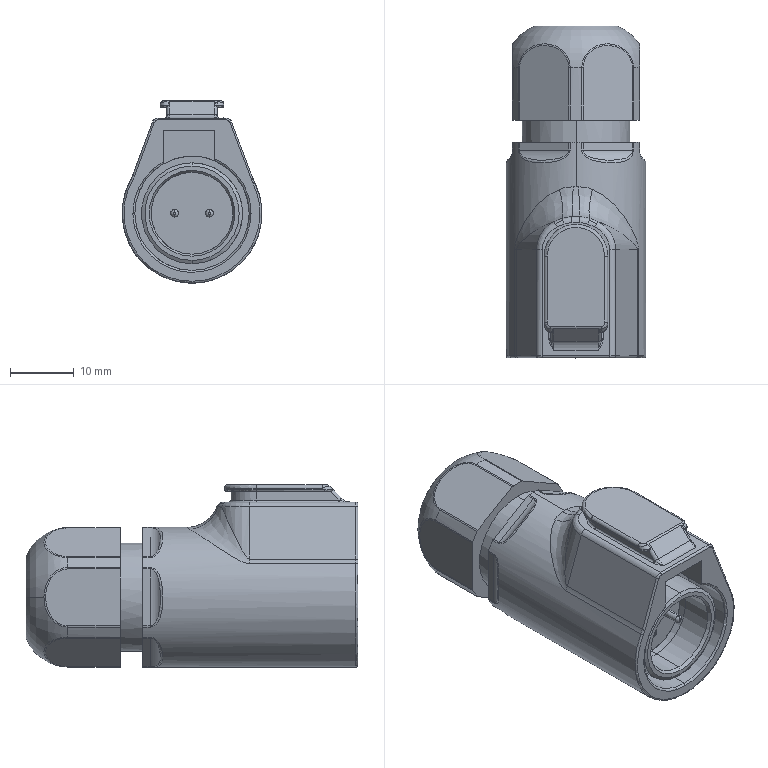Part | SolidWorks | features BaseBody 1 | 1 solid | 179 faces | box 22 x 52.238 x 28.7 mm | volume 17420 mm3 | cylinder 86 | plane 37 | spline 28 | torus 24 | cone 4 | commonest cylinder face diameters 1 x29 22 x9 0.6 x7 4 x7 2 x6 10 x5